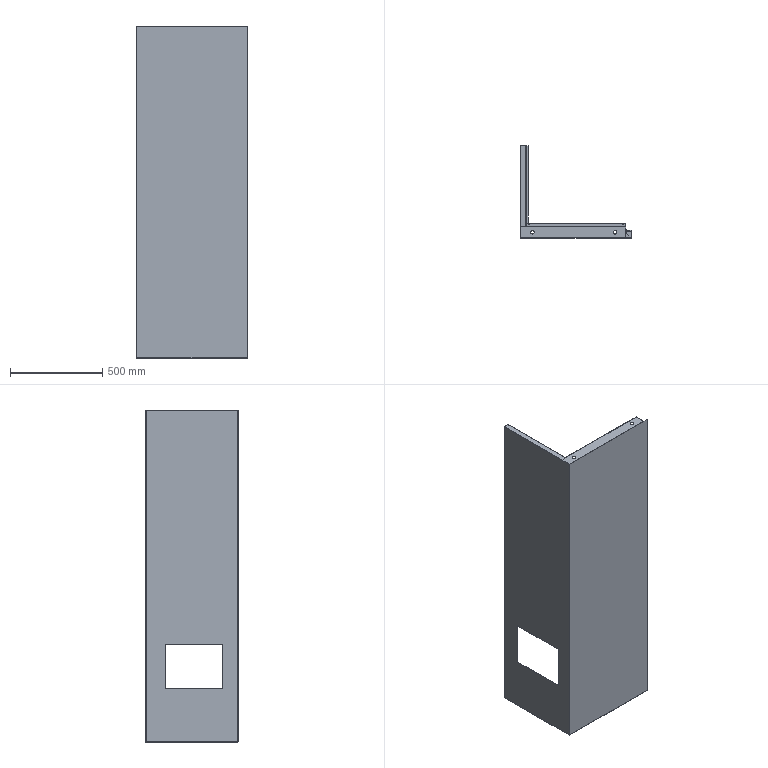Part | STEP file | 1 solid | 156 faces | box 600.001 x 500.001 x 1800 mm | volume 2178717 mm3 | plane 105 | cylinder 46 | spline 5 | commonest cylinder face diameters 0.4 x15 2.4 x15 18 x12 19 x4